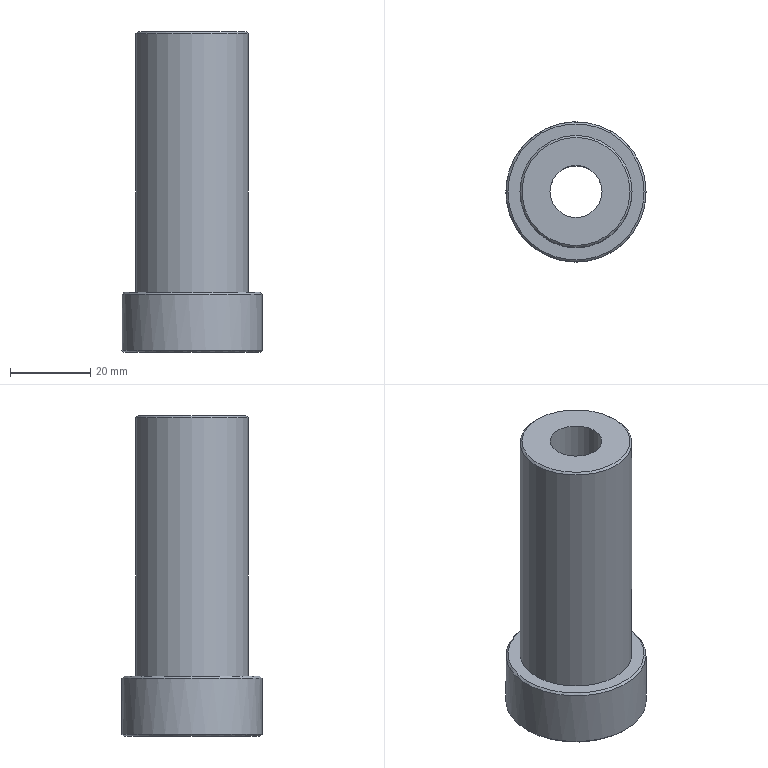Part | STEP file | 车灯-后视镜_id482_x_t | 1 solid | 12 faces | box 35 x 35 x 80 mm | volume 41432 mm3 | plane 4 | cylinder 4 | cone 4 | commonest cylinder face diameters 13 x1 20 x1 28 x1 35 x1
STEP:
#1=CARTESIAN_POINT('',(73.5,-205.,-285.5));
#2=VERTEX_POINT('',#1);
#3=CARTESIAN_POINT('',(60.,-205.,-285.5));
#4=DIRECTION('',(0.,0.,1.));
#5=DIRECTION('',(1.,0.,0.));
#6=AXIS2_PLACEMENT_3D('',#3,#4,#5);
#7=CIRCLE('',#6,13.5);
#8=EDGE_CURVE('',#2,#2,#7,.T.);
#9=ORIENTED_EDGE('',*,*,#8,.T.);
#10=EDGE_LOOP('',(#9));
#11=FACE_BOUND('',#10,.T.);
#12=CARTESIAN_POINT('',(53.5,-205.,-285.5));
#13=VERTEX_POINT('',#12);
#14=CARTESIAN_POINT('',(60.,-205.,-285.5));
#15=DIRECTION('',(0.,0.,-1.));
#16=DIRECTION('',(-1.,0.,0.));
#17=AXIS2_PLACEMENT_3D('',#14,#15,#16);
#18=CIRCLE('',#17,6.5);
#19=EDGE_CURVE('',#13,#13,#18,.T.);
#20=ORIENTED_EDGE('',*,*,#19,.T.);
#21=EDGE_LOOP('',(#20));
#22=FACE_BOUND('',#21,.T.);
#23=CARTESIAN_POINT('',(60.,-205.,-285.5));
#24=DIRECTION('',(0.,0.,1.));
#25=DIRECTION('',(1.,0.,0.));
#26=AXIS2_PLACEMENT_3D('',#23,#24,#25);
#27=PLANE('',#26);
#28=ADVANCED_FACE('',(#11,#22),#27,.T.);
#29=CARTESIAN_POINT('',(74.,-205.,-286.));
#30=VERTEX_POINT('',#29);
#31=CARTESIAN_POINT('',(60.,-205.,-286.));
#32=DIRECTION('',(0.,0.,-1.));
#33=DIRECTION('',(1.,0.,0.));
#34=AXIS2_PLACEMENT_3D('',#31,#32,#33);
#35=CIRCLE('',#34,14.);
#36=EDGE_CURVE('',#30,#30,#35,.T.);
#37=ORIENTED_EDGE('',*,*,#36,.T.);
#38=EDGE_LOOP('',(#37));
#39=FACE_BOUND('',#38,.T.);
#40=CARTESIAN_POINT('',(74.,-205.,-350.5));
#41=VERTEX_POINT('',#40);
#42=CARTESIAN_POINT('',(60.,-205.,-350.5));
#43=DIRECTION('',(0.,0.,-1.));
#44=DIRECTION('',(1.,0.,0.));
#45=AXIS2_PLACEMENT_3D('',#42,#43,#44);
#46=CIRCLE('',#45,14.);
#47=EDGE_CURVE('',#41,#41,#46,.T.);
#48=ORIENTED_EDGE('',*,*,#47,.F.);
#49=EDGE_LOOP('',(#48));
#50=FACE_BOUND('',#49,.T.);
#51=CARTESIAN_POINT('',(60.,-205.,-365.5));
#52=DIRECTION('',(0.,0.,1.));
#53=DIRECTION('',(1.,0.,0.));
#54=AXIS2_PLACEMENT_3D('',#51,#52,#53);
#55=CYLINDRICAL_SURFACE('',#54,14.);
#56=ADVANCED_FACE('',(#39,#50),#55,.T.);
#57=CARTESIAN_POINT('',(77.,-205.,-350.5));
#58=VERTEX_POINT('',#57);
#59=CARTESIAN_POINT('',(60.,-205.,-350.5));
#60=DIRECTION('',(0.,0.,1.));
#61=DIRECTION('',(1.,0.,0.));
#62=AXIS2_PLACEMENT_3D('',#59,#60,#61);
#63=CIRCLE('',#62,17.);
#64=EDGE_CURVE('',#58,#58,#63,.T.);
#65=ORIENTED_EDGE('',*,*,#64,.T.);
#66=EDGE_LOOP('',(#65));
#67=FACE_BOUND('',#66,.T.);
#68=ORIENTED_EDGE('',*,*,#47,.T.);
#69=EDGE_LOOP('',(#68));
#70=FACE_BOUND('',#69,.T.);
#71=CARTESIAN_POINT('',(60.,-205.,-350.5));
#72=DIRECTION('',(0.,0.,1.));
#73=DIRECTION('',(1.,0.,0.));
#74=AXIS2_PLACEMENT_3D('',#71,#72,#73);
#75=PLANE('',#74);
#76=ADVANCED_FACE('',(#67,#70),#75,.T.);
#77=CARTESIAN_POINT('',(77.5,-205.,-351.));
#78=VERTEX_POINT('',#77);
#79=CARTESIAN_POINT('',(60.,-205.,-351.));
#80=DIRECTION('',(0.,0.,-1.));
#81=DIRECTION('',(1.,0.,0.));
#82=AXIS2_PLACEMENT_3D('',#79,#80,#81);
#83=CIRCLE('',#82,17.5);
#84=EDGE_CURVE('',#78,#78,#83,.T.);
#85=ORIENTED_EDGE('',*,*,#84,.T.);
#86=EDGE_LOOP('',(#85));
#87=FACE_BOUND('',#86,.T.);
#88=CARTESIAN_POINT('',(42.5,-205.,-365.));
#89=VERTEX_POINT('',#88);
#90=CARTESIAN_POINT('',(60.,-205.,-365.));
#91=DIRECTION('',(0.,0.,1.));
#92=DIRECTION('',(-1.,0.,0.));
#93=AXIS2_PLACEMENT_3D('',#90,#91,#92);
#94=CIRCLE('',#93,17.5);
#95=EDGE_CURVE('',#89,#89,#94,.T.);
#96=ORIENTED_EDGE('',*,*,#95,.T.);
#97=EDGE_LOOP('',(#96));
#98=FACE_BOUND('',#97,.T.);
#99=CARTESIAN_POINT('',(60.,-205.,-365.5));
#100=DIRECTION('',(0.,0.,1.));
#101=DIRECTION('',(1.,0.,0.));
#102=AXIS2_PLACEMENT_3D('',#99,#100,#101);
#103=CYLINDRICAL_SURFACE('',#102,17.5);
#104=ADVANCED_FACE('',(#87,#98),#103,.T.);
#105=CARTESIAN_POINT('',(49.5,-205.,-365.5));
#106=VERTEX_POINT('',#105);
#107=CARTESIAN_POINT('',(60.,-205.,-365.5));
#108=DIRECTION('',(0.,0.,1.));
#109=DIRECTION('',(-1.,0.,0.));
#110=AXIS2_PLACEMENT_3D('',#107,#108,#109);
#111=CIRCLE('',#110,10.5);
#112=EDGE_CURVE('',#106,#106,#111,.T.);
#113=ORIENTED_EDGE('',*,*,#112,.T.);
#114=EDGE_LOOP('',(#113));
#115=FACE_BOUND('',#114,.T.);
#116=CARTESIAN_POINT('',(43.,-205.,-365.5));
#117=VERTEX_POINT('',#116);
#118=CARTESIAN_POINT('',(60.,-205.,-365.5));
#119=DIRECTION('',(0.,0.,-1.));
#120=DIRECTION('',(-1.,0.,0.));
#121=AXIS2_PLACEMENT_3D('',#118,#119,#120);
#122=CIRCLE('',#121,17.);
#123=EDGE_CURVE('',#117,#117,#122,.T.);
#124=ORIENTED_EDGE('',*,*,#123,.T.);
#125=EDGE_LOOP('',(#124));
#126=FACE_BOUND('',#125,.T.);
#127=CARTESIAN_POINT('',(60.,-205.,-365.5));
#128=DIRECTION('',(0.,0.,-1.));
#129=DIRECTION('',(-1.,0.,0.));
#130=AXIS2_PLACEMENT_3D('',#127,#128,#129);
#131=PLANE('',#130);
#132=ADVANCED_FACE('',(#115,#126),#131,.T.);
#133=CARTESIAN_POINT('',(66.5,-205.,-352.5));
#134=VERTEX_POINT('',#133);
#135=CARTESIAN_POINT('',(60.,-205.,-352.5));
#136=DIRECTION('',(0.,0.,-1.));
#137=DIRECTION('',(1.,0.,0.));
#138=AXIS2_PLACEMENT_3D('',#135,#136,#137);
#139=CIRCLE('',#138,6.5);
#140=EDGE_CURVE('',#134,#134,#139,.T.);
#141=ORIENTED_EDGE('',*,*,#140,.T.);
#142=EDGE_LOOP('',(#141));
#143=FACE_BOUND('',#142,.T.);
#144=ORIENTED_EDGE('',*,*,#19,.F.);
#145=EDGE_LOOP('',(#144));
#146=FACE_BOUND('',#145,.T.);
#147=CARTESIAN_POINT('',(60.,-205.,-285.5));
#148=DIRECTION('',(0.,0.,-1.));
#149=DIRECTION('',(-1.,0.,0.));
#150=AXIS2_PLACEMENT_3D('',#147,#148,#149);
#151=CYLINDRICAL_SURFACE('',#150,6.5);
#152=ADVANCED_FACE('',(#143,#146),#151,.F.);
#153=ORIENTED_EDGE('',*,*,#140,.F.);
#154=EDGE_LOOP('',(#153));
#155=FACE_BOUND('',#154,.T.);
#156=CARTESIAN_POINT('',(50.,-205.,-352.5));
#157=VERTEX_POINT('',#156);
#158=CARTESIAN_POINT('',(60.,-205.,-352.5));
#159=DIRECTION('',(0.,0.,-1.));
#160=DIRECTION('',(-1.,0.,0.));
#161=AXIS2_PLACEMENT_3D('',#158,#159,#160);
#162=CIRCLE('',#161,10.);
#163=EDGE_CURVE('',#157,#157,#162,.T.);
#164=ORIENTED_EDGE('',*,*,#163,.T.);
#165=EDGE_LOOP('',(#164));
#166=FACE_BOUND('',#165,.T.);
#167=CARTESIAN_POINT('',(60.,-205.,-352.5));
#168=DIRECTION('',(0.,0.,1.));
#169=DIRECTION('',(1.,0.,0.));
#170=AXIS2_PLACEMENT_3D('',#167,#168,#169);
#171=PLANE('',#170);
#172=ADVANCED_FACE('',(#155,#166),#171,.F.);
#173=CARTESIAN_POINT('',(50.,-205.,-365.));
#174=VERTEX_POINT('',#173);
#175=CARTESIAN_POINT('',(60.,-205.,-365.));
#176=DIRECTION('',(0.,0.,-1.));
#177=DIRECTION('',(-1.,0.,0.));
#178=AXIS2_PLACEMENT_3D('',#175,#176,#177);
#179=CIRCLE('',#178,10.);
#180=EDGE_CURVE('',#174,#174,#179,.T.);
#181=ORIENTED_EDGE('',*,*,#180,.T.);
#182=EDGE_LOOP('',(#181));
#183=FACE_BOUND('',#182,.T.);
#184=ORIENTED_EDGE('',*,*,#163,.F.);
#185=EDGE_LOOP('',(#184));
#186=FACE_BOUND('',#185,.T.);
#187=CARTESIAN_POINT('',(60.,-205.,-365.5));
#188=DIRECTION('',(0.,0.,1.));
#189=DIRECTION('',(1.,0.,0.));
#190=AXIS2_PLACEMENT_3D('',#187,#188,#189);
#191=CYLINDRICAL_SURFACE('',#190,10.);
#192=ADVANCED_FACE('',(#183,#186),#191,.F.);
#193=ORIENTED_EDGE('',*,*,#180,.F.);
#194=EDGE_LOOP('',(#193));
#195=FACE_BOUND('',#194,.T.);
#196=ORIENTED_EDGE('',*,*,#112,.F.);
#197=EDGE_LOOP('',(#196));
#198=FACE_BOUND('',#197,.T.);
#199=CARTESIAN_POINT('',(60.,-205.,-365.5));
#200=DIRECTION('',(0.,0.,-1.));
#201=DIRECTION('',(-1.,0.,0.));
#202=AXIS2_PLACEMENT_3D('',#199,#200,#201);
#203=CONICAL_SURFACE('',#202,10.5,45.);
#204=ADVANCED_FACE('',(#195,#198),#203,.F.);
#205=ORIENTED_EDGE('',*,*,#64,.F.);
#206=EDGE_LOOP('',(#205));
#207=FACE_BOUND('',#206,.T.);
#208=ORIENTED_EDGE('',*,*,#84,.F.);
#209=EDGE_LOOP('',(#208));
#210=FACE_BOUND('',#209,.T.);
#211=CARTESIAN_POINT('',(60.,-205.,-351.));
#212=DIRECTION('',(0.,0.,-1.));
#213=DIRECTION('',(-1.,0.,0.));
#214=AXIS2_PLACEMENT_3D('',#211,#212,#213);
#215=CONICAL_SURFACE('',#214,17.5,45.);
#216=ADVANCED_FACE('',(#207,#210),#215,.T.);
#217=ORIENTED_EDGE('',*,*,#8,.F.);
#218=EDGE_LOOP('',(#217));
#219=FACE_BOUND('',#218,.T.);
#220=ORIENTED_EDGE('',*,*,#36,.F.);
#221=EDGE_LOOP('',(#220));
#222=FACE_BOUND('',#221,.T.);
#223=CARTESIAN_POINT('',(60.,-205.,-286.));
#224=DIRECTION('',(0.,0.,-1.));
#225=DIRECTION('',(-1.,0.,0.));
#226=AXIS2_PLACEMENT_3D('',#223,#224,#225);
#227=CONICAL_SURFACE('',#226,14.,45.);
#228=ADVANCED_FACE('',(#219,#222),#227,.T.);
#229=ORIENTED_EDGE('',*,*,#123,.F.);
#230=EDGE_LOOP('',(#229));
#231=FACE_BOUND('',#230,.T.);
#232=ORIENTED_EDGE('',*,*,#95,.F.);
#233=EDGE_LOOP('',(#232));
#234=FACE_BOUND('',#233,.T.);
#235=CARTESIAN_POINT('',(60.,-205.,-365.));
#236=DIRECTION('',(0.,0.,1.));
#237=DIRECTION('',(1.,0.,0.));
#238=AXIS2_PLACEMENT_3D('',#235,#236,#237);
#239=CONICAL_SURFACE('',#238,17.5,45.);
#240=ADVANCED_FACE('',(#231,#234),#239,.T.);
#241=CLOSED_SHELL('',(#28,#56,#76,#104,#132,#152,#172,#192,#204,#216,#228,#240));
#242=MANIFOLD_SOLID_BREP('',#241);
#243=(LENGTH_UNIT()NAMED_UNIT(*)SI_UNIT(.MILLI.,.METRE.));
#244=UNCERTAINTY_MEASURE_WITH_UNIT(LENGTH_MEASURE(0.00002),#243,'','');
#245=(NAMED_UNIT(*)PLANE_ANGLE_UNIT()SI_UNIT($,.RADIAN.));
#246=PLANE_ANGLE_MEASURE_WITH_UNIT(PLANE_ANGLE_MEASURE(0.01745),#245);
#247=DIMENSIONAL_EXPONENTS(0.,0.,0.,0.,0.,0.,0.);
#248=(CONVERSION_BASED_UNIT('DEGREE',#246)NAMED_UNIT(#247)PLANE_ANGLE_UNIT());
#249=(NAMED_UNIT(*)SI_UNIT($,.STERADIAN.)SOLID_ANGLE_UNIT());
#250=(GEOMETRIC_REPRESENTATION_CONTEXT(3)GLOBAL_UNCERTAINTY_ASSIGNED_CONTEXT((#244))GLOBAL_UNIT_ASSIGNED_CONTEXT((#243,#248,#249))REPRESENTATION_CONTEXT('',''));
#251=ADVANCED_BREP_SHAPE_REPRESENTATION('',(#242),#250);